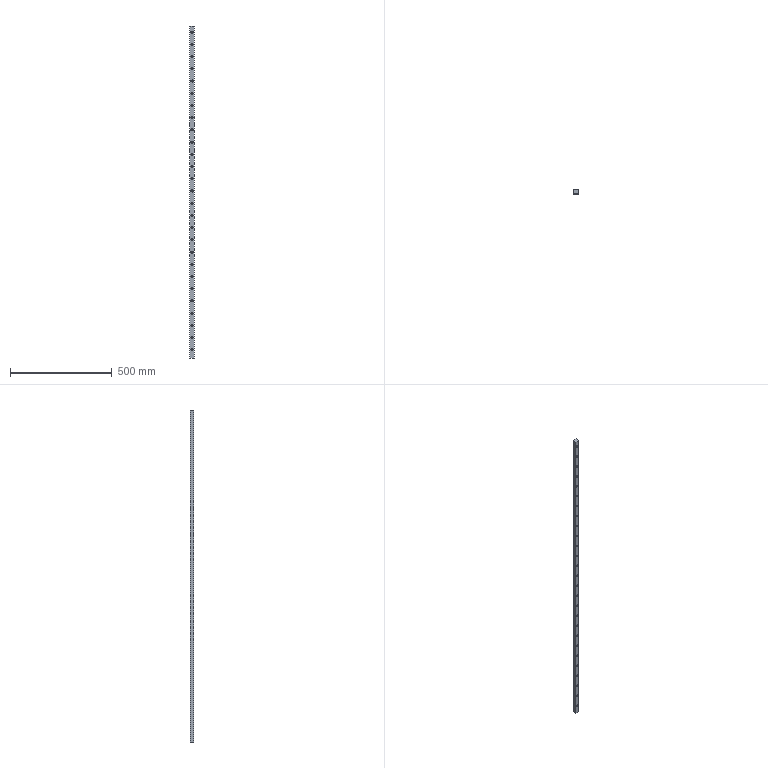Part | SolidWorks | features Extrusion 1, HoleWzd 1, LPattern 1 | 1 solid | 141 faces | box 20 x 17.5 x 1630 mm | volume 550843 mm3 | cylinder 108 | plane 33 | commonest cylinder face diameters 5.5 x54 10 x54